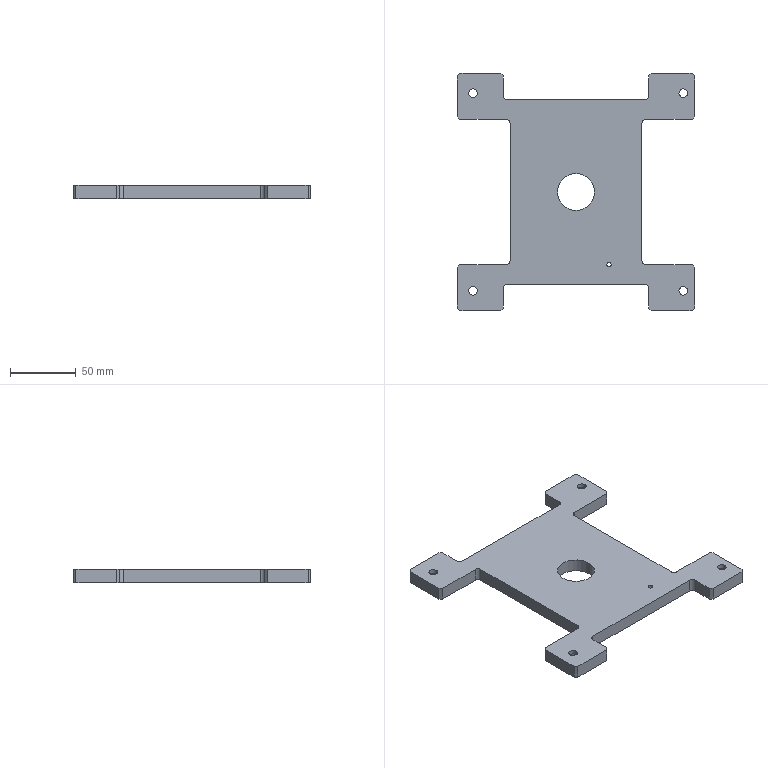Part | SolidWorks | features HoleWzd 2, Chamfer 1, Cut 1, Extrusion 1, Fillet 1 | 1 solid | 66 faces | box 180 x 180 x 10 mm | volume 182649 mm3 | plane 38 | cylinder 28 | commonest cylinder face diameters 6 x8 6.6 x8 11 x8 3.3 x2 28 x2